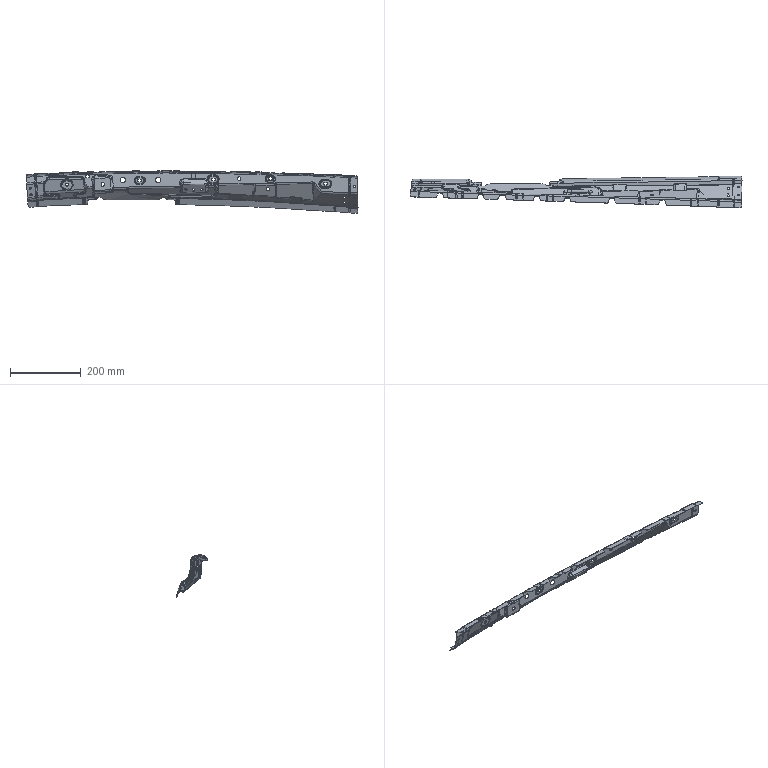Part | STEP file | FNA5401572 | 1 solid | 1598 faces | box 935.734 x 89.628 x 121.004 mm | volume 119341 mm3 | spline 1373 | cylinder 118 | plane 66 | other 29 | sphere 12 | commonest cylinder face diameters 6 x23 8 x20 10 x15 12 x14 7 x12 10.5 x8